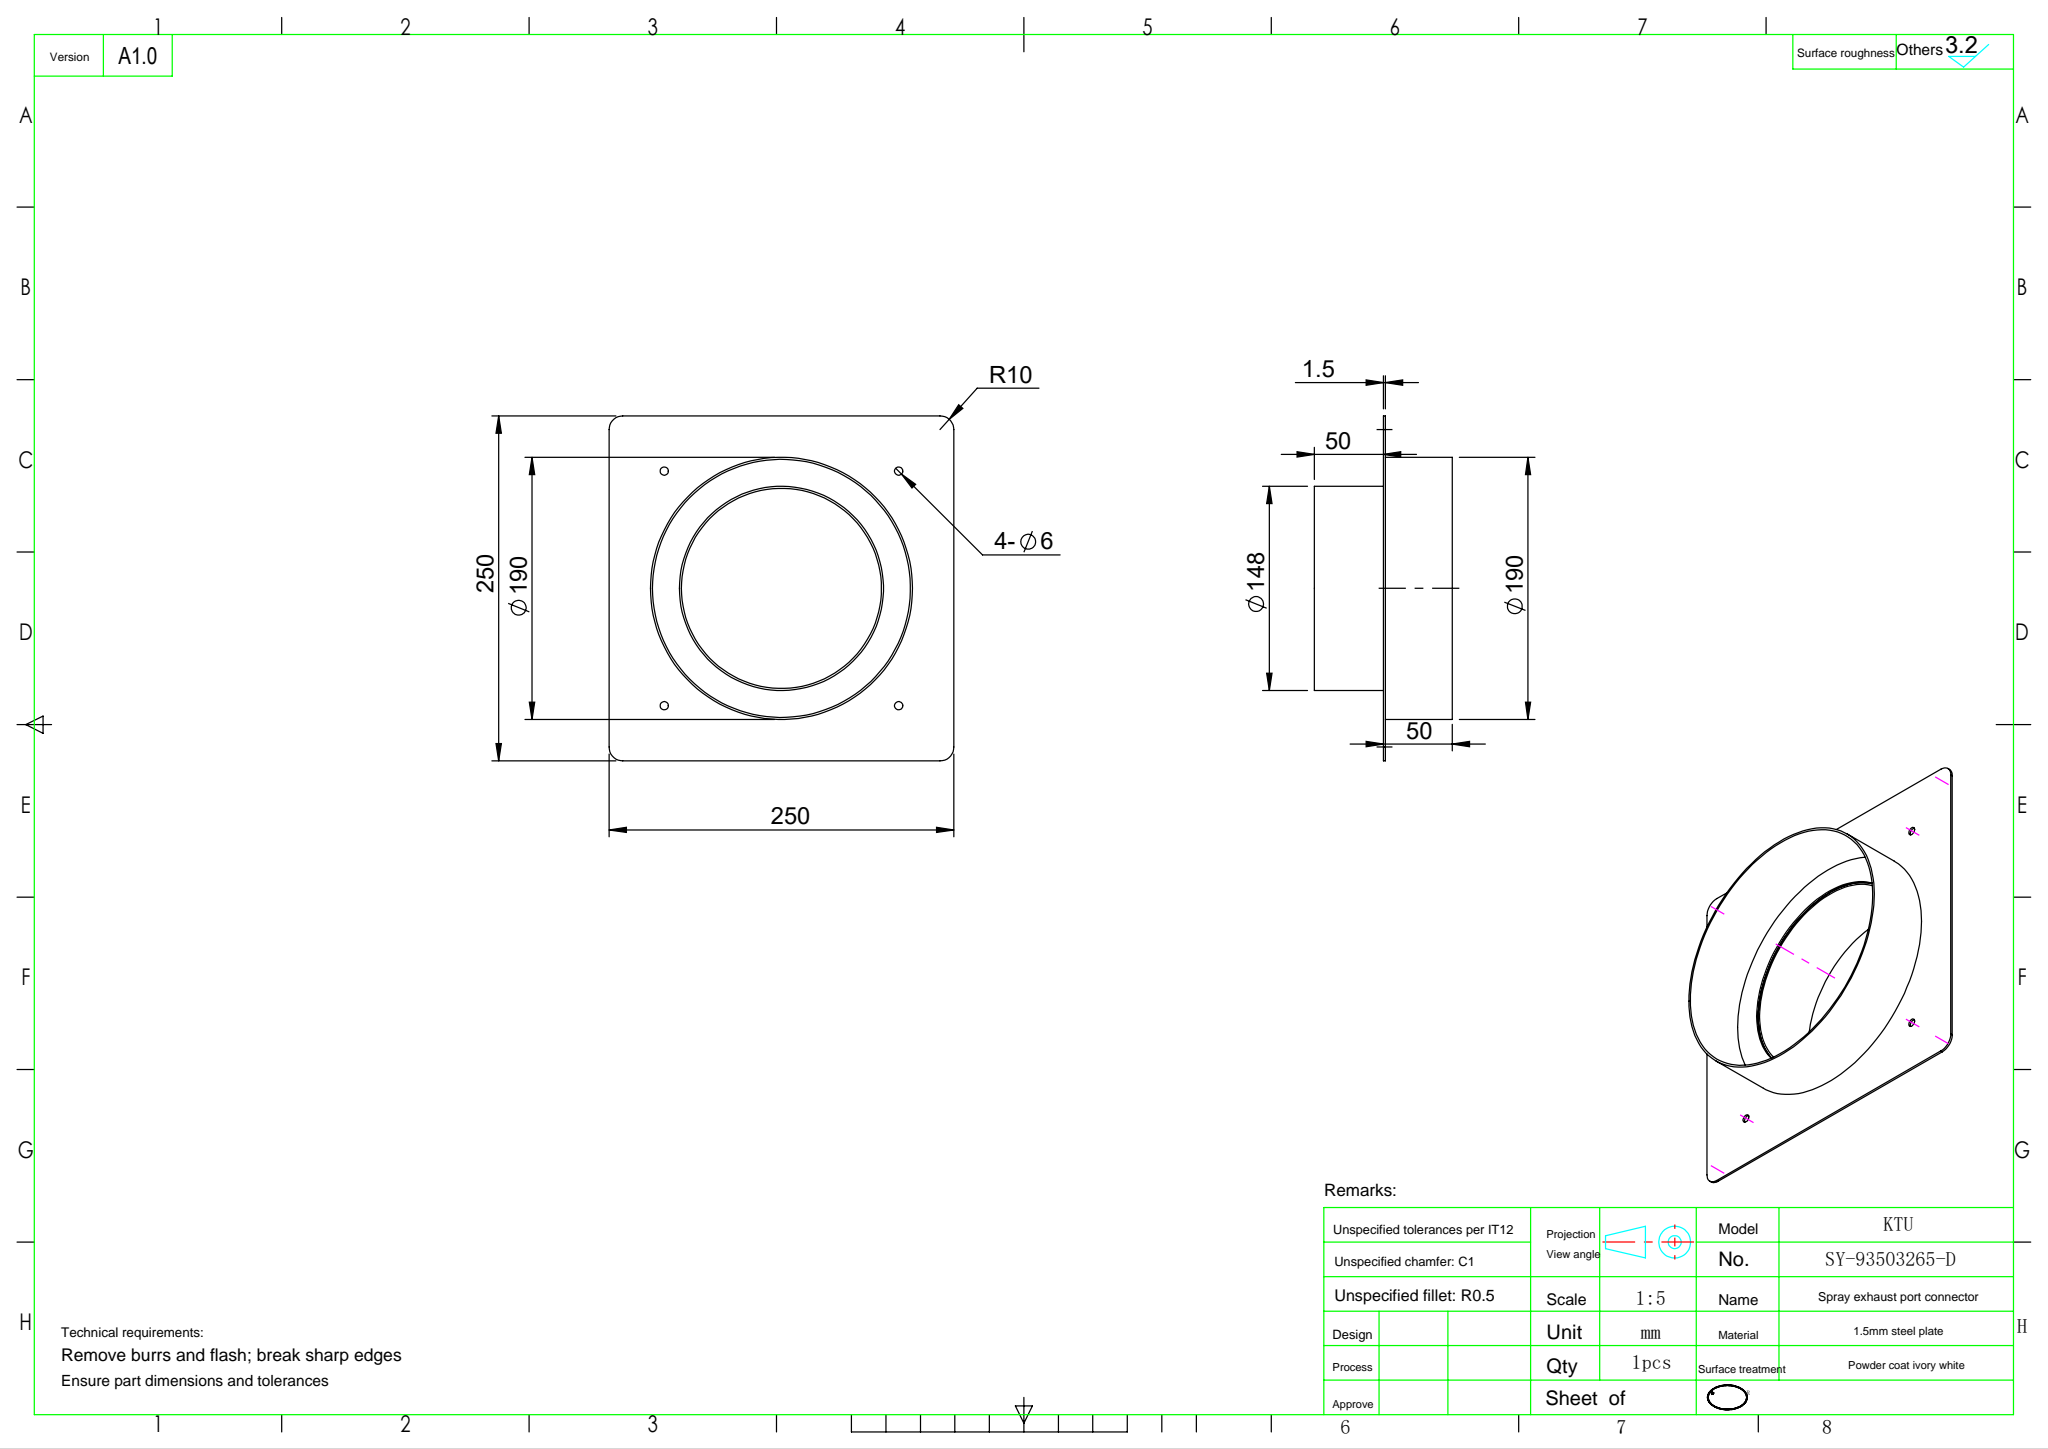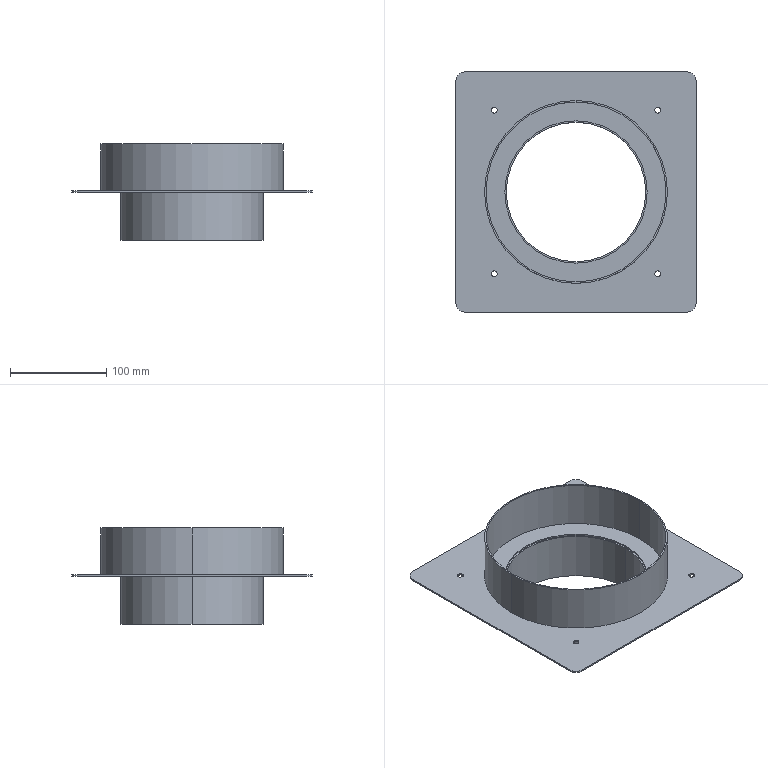Part | SolidWorks | features ICE 4, FlatPattern 1, SMBaseFlange 1, SheetMetal 1 | 2 solids | 32 faces | box 250 x 250 x 100 mm | volume 145247 mm3 | cylinder 22 | plane 10 | commonest cylinder face diameters 6 x8 20 x4 148 x4 145 x2 187 x2 190 x2
STEP:
#1=CARTESIAN_POINT('',(74.,0.,0.));
#2=VERTEX_POINT('',#1);
#3=CARTESIAN_POINT('',(-74.,0.,0.));
#4=VERTEX_POINT('',#3);
#5=CARTESIAN_POINT('',(0.,0.,0.));
#6=DIRECTION('',(0.,0.,-1.));
#7=DIRECTION('',(-1.,0.,0.));
#8=AXIS2_PLACEMENT_3D('',#5,#6,#7);
#9=CIRCLE('',#8,74.);
#10=EDGE_CURVE('',#2,#4,#9,.T.);
#11=ORIENTED_EDGE('',*,*,#10,.F.);
#12=CARTESIAN_POINT('',(74.,0.,-1.5));
#13=VERTEX_POINT('',#12);
#14=CARTESIAN_POINT('',(74.,0.,0.));
#15=DIRECTION('',(0.,0.,-1.));
#16=VECTOR('',#15,1000.);
#17=LINE('',#14,#16);
#18=EDGE_CURVE('',#2,#13,#17,.T.);
#19=ORIENTED_EDGE('',*,*,#18,.T.);
#20=CARTESIAN_POINT('',(-74.,0.,-1.5));
#21=VERTEX_POINT('',#20);
#22=CARTESIAN_POINT('',(0.,0.,-1.5));
#23=DIRECTION('',(0.,0.,-1.));
#24=DIRECTION('',(-1.,0.,0.));
#25=AXIS2_PLACEMENT_3D('',#22,#23,#24);
#26=CIRCLE('',#25,74.);
#27=EDGE_CURVE('',#13,#21,#26,.T.);
#28=ORIENTED_EDGE('',*,*,#27,.T.);
#29=CARTESIAN_POINT('',(-74.,0.,0.));
#30=DIRECTION('',(0.,0.,-1.));
#31=VECTOR('',#30,1000.);
#32=LINE('',#29,#31);
#33=EDGE_CURVE('',#4,#21,#32,.T.);
#34=ORIENTED_EDGE('',*,*,#33,.F.);
#35=EDGE_LOOP('',(#11,#19,#28,#34));
#36=FACE_OUTER_BOUND('',#35,.T.);
#37=CARTESIAN_POINT('',(0.,0.,0.));
#38=DIRECTION('',(0.,0.,-1.));
#39=DIRECTION('',(-1.,0.,0.));
#40=AXIS2_PLACEMENT_3D('',#37,#38,#39);
#41=CYLINDRICAL_SURFACE('',#40,74.);
#42=ADVANCED_FACE('',(#36),#41,.F.);
#43=CARTESIAN_POINT('',(82.,85.,0.));
#44=VERTEX_POINT('',#43);
#45=CARTESIAN_POINT('',(88.,85.,0.));
#46=VERTEX_POINT('',#45);
#47=CARTESIAN_POINT('',(85.,85.,0.));
#48=DIRECTION('',(0.,0.,1.));
#49=DIRECTION('',(1.,0.,0.));
#50=AXIS2_PLACEMENT_3D('',#47,#48,#49);
#51=CIRCLE('',#50,3.);
#52=EDGE_CURVE('',#44,#46,#51,.T.);
#53=ORIENTED_EDGE('',*,*,#52,.T.);
#54=CARTESIAN_POINT('',(88.,85.,-1.5));
#55=VERTEX_POINT('',#54);
#56=CARTESIAN_POINT('',(88.,85.,46.5));
#57=DIRECTION('',(0.,0.,-1.));
#58=VECTOR('',#57,1000.);
#59=LINE('',#56,#58);
#60=EDGE_CURVE('',#46,#55,#59,.T.);
#61=ORIENTED_EDGE('',*,*,#60,.T.);
#62=CARTESIAN_POINT('',(82.,85.,-1.5));
#63=VERTEX_POINT('',#62);
#64=CARTESIAN_POINT('',(85.,85.,-1.5));
#65=DIRECTION('',(0.,0.,-1.));
#66=DIRECTION('',(-1.,0.,0.));
#67=AXIS2_PLACEMENT_3D('',#64,#65,#66);
#68=CIRCLE('',#67,3.);
#69=EDGE_CURVE('',#55,#63,#68,.T.);
#70=ORIENTED_EDGE('',*,*,#69,.T.);
#71=CARTESIAN_POINT('',(82.,85.,46.5));
#72=DIRECTION('',(0.,0.,-1.));
#73=VECTOR('',#72,1000.);
#74=LINE('',#71,#73);
#75=EDGE_CURVE('',#44,#63,#74,.T.);
#76=ORIENTED_EDGE('',*,*,#75,.F.);
#77=EDGE_LOOP('',(#53,#61,#70,#76));
#78=FACE_OUTER_BOUND('',#77,.T.);
#79=CARTESIAN_POINT('',(85.,85.,46.5));
#80=DIRECTION('',(0.,0.,-1.));
#81=DIRECTION('',(-1.,0.,0.));
#82=AXIS2_PLACEMENT_3D('',#79,#80,#81);
#83=CYLINDRICAL_SURFACE('',#82,3.);
#84=ADVANCED_FACE('',(#78),#83,.F.);
#85=CARTESIAN_POINT('',(82.,-85.,0.));
#86=VERTEX_POINT('',#85);
#87=CARTESIAN_POINT('',(88.,-85.,0.));
#88=VERTEX_POINT('',#87);
#89=CARTESIAN_POINT('',(85.,-85.,0.));
#90=DIRECTION('',(0.,0.,1.));
#91=DIRECTION('',(1.,0.,0.));
#92=AXIS2_PLACEMENT_3D('',#89,#90,#91);
#93=CIRCLE('',#92,3.);
#94=EDGE_CURVE('',#86,#88,#93,.T.);
#95=ORIENTED_EDGE('',*,*,#94,.T.);
#96=CARTESIAN_POINT('',(88.,-85.,-1.5));
#97=VERTEX_POINT('',#96);
#98=CARTESIAN_POINT('',(88.,-85.,46.5));
#99=DIRECTION('',(0.,0.,-1.));
#100=VECTOR('',#99,1000.);
#101=LINE('',#98,#100);
#102=EDGE_CURVE('',#88,#97,#101,.T.);
#103=ORIENTED_EDGE('',*,*,#102,.T.);
#104=CARTESIAN_POINT('',(82.,-85.,-1.5));
#105=VERTEX_POINT('',#104);
#106=CARTESIAN_POINT('',(85.,-85.,-1.5));
#107=DIRECTION('',(0.,0.,-1.));
#108=DIRECTION('',(-1.,0.,0.));
#109=AXIS2_PLACEMENT_3D('',#106,#107,#108);
#110=CIRCLE('',#109,3.);
#111=EDGE_CURVE('',#97,#105,#110,.T.);
#112=ORIENTED_EDGE('',*,*,#111,.T.);
#113=CARTESIAN_POINT('',(82.,-85.,46.5));
#114=DIRECTION('',(0.,0.,-1.));
#115=VECTOR('',#114,1000.);
#116=LINE('',#113,#115);
#117=EDGE_CURVE('',#86,#105,#116,.T.);
#118=ORIENTED_EDGE('',*,*,#117,.F.);
#119=EDGE_LOOP('',(#95,#103,#112,#118));
#120=FACE_OUTER_BOUND('',#119,.T.);
#121=CARTESIAN_POINT('',(85.,-85.,46.5));
#122=DIRECTION('',(0.,0.,-1.));
#123=DIRECTION('',(-1.,0.,0.));
#124=AXIS2_PLACEMENT_3D('',#121,#122,#123);
#125=CYLINDRICAL_SURFACE('',#124,3.);
#126=ADVANCED_FACE('',(#120),#125,.F.);
#127=CARTESIAN_POINT('',(-88.,-85.,0.));
#128=VERTEX_POINT('',#127);
#129=CARTESIAN_POINT('',(-82.,-85.,0.));
#130=VERTEX_POINT('',#129);
#131=CARTESIAN_POINT('',(-85.,-85.,0.));
#132=DIRECTION('',(0.,0.,1.));
#133=DIRECTION('',(1.,0.,0.));
#134=AXIS2_PLACEMENT_3D('',#131,#132,#133);
#135=CIRCLE('',#134,3.);
#136=EDGE_CURVE('',#128,#130,#135,.T.);
#137=ORIENTED_EDGE('',*,*,#136,.T.);
#138=CARTESIAN_POINT('',(-82.,-85.,-1.5));
#139=VERTEX_POINT('',#138);
#140=CARTESIAN_POINT('',(-82.,-85.,46.5));
#141=DIRECTION('',(0.,0.,-1.));
#142=VECTOR('',#141,1000.);
#143=LINE('',#140,#142);
#144=EDGE_CURVE('',#130,#139,#143,.T.);
#145=ORIENTED_EDGE('',*,*,#144,.T.);
#146=CARTESIAN_POINT('',(-88.,-85.,-1.5));
#147=VERTEX_POINT('',#146);
#148=CARTESIAN_POINT('',(-85.,-85.,-1.5));
#149=DIRECTION('',(0.,0.,-1.));
#150=DIRECTION('',(-1.,0.,0.));
#151=AXIS2_PLACEMENT_3D('',#148,#149,#150);
#152=CIRCLE('',#151,3.);
#153=EDGE_CURVE('',#139,#147,#152,.T.);
#154=ORIENTED_EDGE('',*,*,#153,.T.);
#155=CARTESIAN_POINT('',(-88.,-85.,46.5));
#156=DIRECTION('',(0.,0.,-1.));
#157=VECTOR('',#156,1000.);
#158=LINE('',#155,#157);
#159=EDGE_CURVE('',#128,#147,#158,.T.);
#160=ORIENTED_EDGE('',*,*,#159,.F.);
#161=EDGE_LOOP('',(#137,#145,#154,#160));
#162=FACE_OUTER_BOUND('',#161,.T.);
#163=CARTESIAN_POINT('',(-85.,-85.,46.5));
#164=DIRECTION('',(0.,0.,-1.));
#165=DIRECTION('',(-1.,0.,0.));
#166=AXIS2_PLACEMENT_3D('',#163,#164,#165);
#167=CYLINDRICAL_SURFACE('',#166,3.);
#168=ADVANCED_FACE('',(#162),#167,.F.);
#169=CARTESIAN_POINT('',(-88.,85.,0.));
#170=VERTEX_POINT('',#169);
#171=CARTESIAN_POINT('',(-82.,85.,0.));
#172=VERTEX_POINT('',#171);
#173=CARTESIAN_POINT('',(-85.,85.,0.));
#174=DIRECTION('',(0.,0.,1.));
#175=DIRECTION('',(1.,0.,0.));
#176=AXIS2_PLACEMENT_3D('',#173,#174,#175);
#177=CIRCLE('',#176,3.);
#178=EDGE_CURVE('',#170,#172,#177,.T.);
#179=ORIENTED_EDGE('',*,*,#178,.T.);
#180=CARTESIAN_POINT('',(-82.,85.,-1.5));
#181=VERTEX_POINT('',#180);
#182=CARTESIAN_POINT('',(-82.,85.,46.5));
#183=DIRECTION('',(0.,0.,-1.));
#184=VECTOR('',#183,1000.);
#185=LINE('',#182,#184);
#186=EDGE_CURVE('',#172,#181,#185,.T.);
#187=ORIENTED_EDGE('',*,*,#186,.T.);
#188=CARTESIAN_POINT('',(-88.,85.,-1.5));
#189=VERTEX_POINT('',#188);
#190=CARTESIAN_POINT('',(-85.,85.,-1.5));
#191=DIRECTION('',(0.,0.,-1.));
#192=DIRECTION('',(-1.,0.,0.));
#193=AXIS2_PLACEMENT_3D('',#190,#191,#192);
#194=CIRCLE('',#193,3.);
#195=EDGE_CURVE('',#181,#189,#194,.T.);
#196=ORIENTED_EDGE('',*,*,#195,.T.);
#197=CARTESIAN_POINT('',(-88.,85.,46.5));
#198=DIRECTION('',(0.,0.,-1.));
#199=VECTOR('',#198,1000.);
#200=LINE('',#197,#199);
#201=EDGE_CURVE('',#170,#189,#200,.T.);
#202=ORIENTED_EDGE('',*,*,#201,.F.);
#203=EDGE_LOOP('',(#179,#187,#196,#202));
#204=FACE_OUTER_BOUND('',#203,.T.);
#205=CARTESIAN_POINT('',(-85.,85.,46.5));
#206=DIRECTION('',(0.,0.,-1.));
#207=DIRECTION('',(-1.,0.,0.));
#208=AXIS2_PLACEMENT_3D('',#205,#206,#207);
#209=CYLINDRICAL_SURFACE('',#208,3.);
#210=ADVANCED_FACE('',(#204),#209,.F.);
#211=CARTESIAN_POINT('',(-95.,0.,48.5));
#212=VERTEX_POINT('',#211);
#213=CARTESIAN_POINT('',(95.,0.,48.5));
#214=VERTEX_POINT('',#213);
#215=CARTESIAN_POINT('',(0.,0.,48.5));
#216=DIRECTION('',(0.,0.,-1.));
#217=DIRECTION('',(-1.,0.,0.));
#218=AXIS2_PLACEMENT_3D('',#215,#216,#217);
#219=CIRCLE('',#218,95.);
#220=EDGE_CURVE('',#212,#214,#219,.T.);
#221=ORIENTED_EDGE('',*,*,#220,.T.);
#222=CARTESIAN_POINT('',(95.,0.,0.));
#223=VERTEX_POINT('',#222);
#224=CARTESIAN_POINT('',(95.,0.,48.5));
#225=DIRECTION('',(0.,0.,-1.));
#226=VECTOR('',#225,1000.);
#227=LINE('',#224,#226);
#228=EDGE_CURVE('',#214,#223,#227,.T.);
#229=ORIENTED_EDGE('',*,*,#228,.T.);
#230=CARTESIAN_POINT('',(-95.,0.,0.));
#231=VERTEX_POINT('',#230);
#232=CARTESIAN_POINT('',(0.,0.,0.));
#233=DIRECTION('',(0.,0.,1.));
#234=DIRECTION('',(1.,0.,0.));
#235=AXIS2_PLACEMENT_3D('',#232,#233,#234);
#236=CIRCLE('',#235,95.);
#237=EDGE_CURVE('',#223,#231,#236,.T.);
#238=ORIENTED_EDGE('',*,*,#237,.T.);
#239=CARTESIAN_POINT('',(-95.,0.,48.5));
#240=DIRECTION('',(0.,0.,-1.));
#241=VECTOR('',#240,1000.);
#242=LINE('',#239,#241);
#243=EDGE_CURVE('',#212,#231,#242,.T.);
#244=ORIENTED_EDGE('',*,*,#243,.F.);
#245=EDGE_LOOP('',(#221,#229,#238,#244));
#246=FACE_OUTER_BOUND('',#245,.T.);
#247=CARTESIAN_POINT('',(0.,0.,48.5));
#248=DIRECTION('',(0.,0.,-1.));
#249=DIRECTION('',(-1.,0.,0.));
#250=AXIS2_PLACEMENT_3D('',#247,#248,#249);
#251=CYLINDRICAL_SURFACE('',#250,95.);
#252=ADVANCED_FACE('',(#246),#251,.T.);
#253=CARTESIAN_POINT('',(93.5,0.,48.5));
#254=VERTEX_POINT('',#253);
#255=CARTESIAN_POINT('',(-93.5,0.,48.5));
#256=VERTEX_POINT('',#255);
#257=CARTESIAN_POINT('',(0.,0.,48.5));
#258=DIRECTION('',(0.,0.,-1.));
#259=DIRECTION('',(-1.,0.,0.));
#260=AXIS2_PLACEMENT_3D('',#257,#258,#259);
#261=CIRCLE('',#260,93.5);
#262=EDGE_CURVE('',#254,#256,#261,.T.);
#263=ORIENTED_EDGE('',*,*,#262,.F.);
#264=CARTESIAN_POINT('',(93.5,0.,0.));
#265=VERTEX_POINT('',#264);
#266=CARTESIAN_POINT('',(93.5,0.,48.5));
#267=DIRECTION('',(0.,0.,-1.));
#268=VECTOR('',#267,1000.);
#269=LINE('',#266,#268);
#270=EDGE_CURVE('',#254,#265,#269,.T.);
#271=ORIENTED_EDGE('',*,*,#270,.T.);
#272=CARTESIAN_POINT('',(-93.5,0.,0.));
#273=VERTEX_POINT('',#272);
#274=CARTESIAN_POINT('',(0.,0.,0.));
#275=DIRECTION('',(0.,0.,1.));
#276=DIRECTION('',(-1.,0.,0.));
#277=AXIS2_PLACEMENT_3D('',#274,#275,#276);
#278=CIRCLE('',#277,93.5);
#279=EDGE_CURVE('',#273,#265,#278,.T.);
#280=ORIENTED_EDGE('',*,*,#279,.F.);
#281=CARTESIAN_POINT('',(-93.5,0.,48.5));
#282=DIRECTION('',(0.,0.,-1.));
#283=VECTOR('',#282,1000.);
#284=LINE('',#281,#283);
#285=EDGE_CURVE('',#256,#273,#284,.T.);
#286=ORIENTED_EDGE('',*,*,#285,.F.);
#287=EDGE_LOOP('',(#263,#271,#280,#286));
#288=FACE_OUTER_BOUND('',#287,.T.);
#289=CARTESIAN_POINT('',(0.,0.,48.5));
#290=DIRECTION('',(0.,0.,-1.));
#291=DIRECTION('',(-1.,0.,0.));
#292=AXIS2_PLACEMENT_3D('',#289,#290,#291);
#293=CYLINDRICAL_SURFACE('',#292,93.5);
#294=ADVANCED_FACE('',(#288),#293,.F.);
#295=ORIENTED_EDGE('',*,*,#270,.F.);
#296=CARTESIAN_POINT('',(0.,0.,48.5));
#297=DIRECTION('',(0.,0.,-1.));
#298=DIRECTION('',(-1.,0.,0.));
#299=AXIS2_PLACEMENT_3D('',#296,#297,#298);
#300=CIRCLE('',#299,93.5);
#301=EDGE_CURVE('',#256,#254,#300,.T.);
#302=ORIENTED_EDGE('',*,*,#301,.F.);
#303=ORIENTED_EDGE('',*,*,#285,.T.);
#304=CARTESIAN_POINT('',(0.,0.,0.));
#305=DIRECTION('',(0.,0.,1.));
#306=DIRECTION('',(-1.,0.,0.));
#307=AXIS2_PLACEMENT_3D('',#304,#305,#306);
#308=CIRCLE('',#307,93.5);
#309=EDGE_CURVE('',#265,#273,#308,.T.);
#310=ORIENTED_EDGE('',*,*,#309,.F.);
#311=EDGE_LOOP('',(#295,#302,#303,#310));
#312=FACE_OUTER_BOUND('',#311,.T.);
#313=CARTESIAN_POINT('',(0.,0.,48.5));
#314=DIRECTION('',(0.,0.,-1.));
#315=DIRECTION('',(-1.,0.,0.));
#316=AXIS2_PLACEMENT_3D('',#313,#314,#315);
#317=CYLINDRICAL_SURFACE('',#316,93.5);
#318=ADVANCED_FACE('',(#312),#317,.F.);
#319=CARTESIAN_POINT('',(-125.,-115.,0.));
#320=VERTEX_POINT('',#319);
#321=CARTESIAN_POINT('',(-115.,-125.,0.));
#322=VERTEX_POINT('',#321);
#323=CARTESIAN_POINT('',(-115.,-115.,0.));
#324=DIRECTION('',(0.,0.,1.));
#325=DIRECTION('',(1.,0.,0.));
#326=AXIS2_PLACEMENT_3D('',#323,#324,#325);
#327=CIRCLE('',#326,10.);
#328=EDGE_CURVE('',#320,#322,#327,.T.);
#329=ORIENTED_EDGE('',*,*,#328,.F.);
#330=CARTESIAN_POINT('',(-125.,-115.,-1.5));
#331=VERTEX_POINT('',#330);
#332=CARTESIAN_POINT('',(-125.,-115.,-1.5));
#333=DIRECTION('',(0.,0.,1.));
#334=VECTOR('',#333,1000.);
#335=LINE('',#332,#334);
#336=EDGE_CURVE('',#331,#320,#335,.T.);
#337=ORIENTED_EDGE('',*,*,#336,.F.);
#338=CARTESIAN_POINT('',(-115.,-125.,-1.5));
#339=VERTEX_POINT('',#338);
#340=CARTESIAN_POINT('',(-115.,-115.,-1.5));
#341=DIRECTION('',(0.,0.,1.));
#342=DIRECTION('',(1.,0.,0.));
#343=AXIS2_PLACEMENT_3D('',#340,#341,#342);
#344=CIRCLE('',#343,10.);
#345=EDGE_CURVE('',#331,#339,#344,.T.);
#346=ORIENTED_EDGE('',*,*,#345,.T.);
#347=CARTESIAN_POINT('',(-115.,-125.,-1.5));
#348=DIRECTION('',(0.,0.,1.));
#349=VECTOR('',#348,1000.);
#350=LINE('',#347,#349);
#351=EDGE_CURVE('',#339,#322,#350,.T.);
#352=ORIENTED_EDGE('',*,*,#351,.T.);
#353=EDGE_LOOP('',(#329,#337,#346,#352));
#354=FACE_OUTER_BOUND('',#353,.T.);
#355=CARTESIAN_POINT('',(-115.,-115.,-1.5));
#356=DIRECTION('',(0.,0.,1.));
#357=DIRECTION('',(1.,0.,0.));
#358=AXIS2_PLACEMENT_3D('',#355,#356,#357);
#359=CYLINDRICAL_SURFACE('',#358,10.);
#360=ADVANCED_FACE('',(#354),#359,.T.);
#361=CARTESIAN_POINT('',(-125.,115.,0.));
#362=VERTEX_POINT('',#361);
#363=CARTESIAN_POINT('',(-125.,-115.,0.));
#364=DIRECTION('',(0.,-1.,0.));
#365=VECTOR('',#364,1000.);
#366=LINE('',#363,#365);
#367=EDGE_CURVE('',#362,#320,#366,.T.);
#368=ORIENTED_EDGE('',*,*,#367,.F.);
#369=CARTESIAN_POINT('',(-125.,115.,-1.5));
#370=VERTEX_POINT('',#369);
#371=CARTESIAN_POINT('',(-125.,115.,-1.5));
#372=DIRECTION('',(0.,0.,1.));
#373=VECTOR('',#372,1000.);
#374=LINE('',#371,#373);
#375=EDGE_CURVE('',#370,#362,#374,.T.);
#376=ORIENTED_EDGE('',*,*,#375,.F.);
#377=CARTESIAN_POINT('',(-125.,-115.,-1.5));
#378=DIRECTION('',(0.,-1.,0.));
#379=VECTOR('',#378,1000.);
#380=LINE('',#377,#379);
#381=EDGE_CURVE('',#370,#331,#380,.T.);
#382=ORIENTED_EDGE('',*,*,#381,.T.);
#383=ORIENTED_EDGE('',*,*,#336,.T.);
#384=EDGE_LOOP('',(#368,#376,#382,#383));
#385=FACE_OUTER_BOUND('',#384,.T.);
#386=CARTESIAN_POINT('',(-125.,-115.,-1.5));
#387=DIRECTION('',(-1.,0.,0.));
#388=DIRECTION('',(0.,0.,1.));
#389=AXIS2_PLACEMENT_3D('',#386,#387,#388);
#390=PLANE('',#389);
#391=ADVANCED_FACE('',(#385),#390,.T.);
#392=CARTESIAN_POINT('',(-115.,125.,0.));
#393=VERTEX_POINT('',#392);
#394=CARTESIAN_POINT('',(-115.,115.,0.));
#395=DIRECTION('',(0.,0.,1.));
#396=DIRECTION('',(-1.,0.,0.));
#397=AXIS2_PLACEMENT_3D('',#394,#395,#396);
#398=CIRCLE('',#397,10.);
#399=EDGE_CURVE('',#393,#362,#398,.T.);
#400=ORIENTED_EDGE('',*,*,#399,.F.);
#401=CARTESIAN_POINT('',(-115.,125.,-1.5));
#402=VERTEX_POINT('',#401);
#403=CARTESIAN_POINT('',(-115.,125.,-1.5));
#404=DIRECTION('',(0.,0.,1.));
#405=VECTOR('',#404,1000.);
#406=LINE('',#403,#405);
#407=EDGE_CURVE('',#402,#393,#406,.T.);
#408=ORIENTED_EDGE('',*,*,#407,.F.);
#409=CARTESIAN_POINT('',(-115.,115.,-1.5));
#410=DIRECTION('',(0.,0.,1.));
#411=DIRECTION('',(-1.,0.,0.));
#412=AXIS2_PLACEMENT_3D('',#409,#410,#411);
#413=CIRCLE('',#412,10.);
#414=EDGE_CURVE('',#402,#370,#413,.T.);
#415=ORIENTED_EDGE('',*,*,#414,.T.);
#416=ORIENTED_EDGE('',*,*,#375,.T.);
#417=EDGE_LOOP('',(#400,#408,#415,#416));
#418=FACE_OUTER_BOUND('',#417,.T.);
#419=CARTESIAN_POINT('',(-115.,115.,-1.5));
#420=DIRECTION('',(0.,0.,1.));
#421=DIRECTION('',(1.,0.,0.));
#422=AXIS2_PLACEMENT_3D('',#419,#420,#421);
#423=CYLINDRICAL_SURFACE('',#422,10.);
#424=ADVANCED_FACE('',(#418),#423,.T.);
#425=CARTESIAN_POINT('',(115.,125.,0.));
#426=VERTEX_POINT('',#425);
#427=CARTESIAN_POINT('',(-115.,125.,0.));
#428=DIRECTION('',(-1.,0.,0.));
#429=VECTOR('',#428,1000.);
#430=LINE('',#427,#429);
#431=EDGE_CURVE('',#426,#393,#430,.T.);
#432=ORIENTED_EDGE('',*,*,#431,.F.);
#433=CARTESIAN_POINT('',(115.,125.,-1.5));
#434=VERTEX_POINT('',#433);
#435=CARTESIAN_POINT('',(115.,125.,-1.5));
#436=DIRECTION('',(0.,0.,1.));
#437=VECTOR('',#436,1000.);
#438=LINE('',#435,#437);
#439=EDGE_CURVE('',#434,#426,#438,.T.);
#440=ORIENTED_EDGE('',*,*,#439,.F.);
#441=CARTESIAN_POINT('',(-115.,125.,-1.5));
#442=DIRECTION('',(-1.,0.,0.));
#443=VECTOR('',#442,1000.);
#444=LINE('',#441,#443);
#445=EDGE_CURVE('',#434,#402,#444,.T.);
#446=ORIENTED_EDGE('',*,*,#445,.T.);
#447=ORIENTED_EDGE('',*,*,#407,.T.);
#448=EDGE_LOOP('',(#432,#440,#446,#447));
#449=FACE_OUTER_BOUND('',#448,.T.);
#450=CARTESIAN_POINT('',(-115.,125.,-1.5));
#451=DIRECTION('',(0.,1.,0.));
#452=DIRECTION('',(0.,0.,1.));
#453=AXIS2_PLACEMENT_3D('',#450,#451,#452);
#454=PLANE('',#453);
#455=ADVANCED_FACE('',(#449),#454,.T.);
#456=CARTESIAN_POINT('',(125.,115.,0.));
#457=VERTEX_POINT('',#456);
#458=CARTESIAN_POINT('',(115.,115.,0.));
#459=DIRECTION('',(0.,0.,1.));
#460=DIRECTION('',(1.,0.,0.));
#461=AXIS2_PLACEMENT_3D('',#458,#459,#460);
#462=CIRCLE('',#461,10.);
#463=EDGE_CURVE('',#457,#426,#462,.T.);
#464=ORIENTED_EDGE('',*,*,#463,.F.);
#465=CARTESIAN_POINT('',(125.,115.,-1.5));
#466=VERTEX_POINT('',#465);
#467=CARTESIAN_POINT('',(125.,115.,-1.5));
#468=DIRECTION('',(0.,0.,1.));
#469=VECTOR('',#468,1000.);
#470=LINE('',#467,#469);
#471=EDGE_CURVE('',#466,#457,#470,.T.);
#472=ORIENTED_EDGE('',*,*,#471,.F.);
#473=CARTESIAN_POINT('',(115.,115.,-1.5));
#474=DIRECTION('',(0.,0.,1.));
#475=DIRECTION('',(1.,0.,0.));
#476=AXIS2_PLACEMENT_3D('',#473,#474,#475);
#477=CIRCLE('',#476,10.);
#478=EDGE_CURVE('',#466,#434,#477,.T.);
#479=ORIENTED_EDGE('',*,*,#478,.T.);
#480=ORIENTED_EDGE('',*,*,#439,.T.);
#481=EDGE_LOOP('',(#464,#472,#479,#480));
#482=FACE_OUTER_BOUND('',#481,.T.);
#483=CARTESIAN_POINT('',(115.,115.,-1.5));
#484=DIRECTION('',(0.,0.,1.));
#485=DIRECTION('',(1.,0.,0.));
#486=AXIS2_PLACEMENT_3D('',#483,#484,#485);
#487=CYLINDRICAL_SURFACE('',#486,10.);
#488=ADVANCED_FACE('',(#482),#487,.T.);
#489=CARTESIAN_POINT('',(125.,-115.,0.));
#490=VERTEX_POINT('',#489);
#491=CARTESIAN_POINT('',(125.,-115.,0.));
#492=DIRECTION('',(0.,1.,0.));
#493=VECTOR('',#492,1000.);
#494=LINE('',#491,#493);
#495=EDGE_CURVE('',#490,#457,#494,.T.);
#496=ORIENTED_EDGE('',*,*,#495,.F.);
#497=CARTESIAN_POINT('',(125.,-115.,-1.5));
#498=VERTEX_POINT('',#497);
#499=CARTESIAN_POINT('',(125.,-115.,-1.5));
#500=DIRECTION('',(0.,0.,1.));
#501=VECTOR('',#500,1000.);
#502=LINE('',#499,#501);
#503=EDGE_CURVE('',#498,#490,#502,.T.);
#504=ORIENTED_EDGE('',*,*,#503,.F.);
#505=CARTESIAN_POINT('',(125.,-115.,-1.5));
#506=DIRECTION('',(0.,1.,0.));
#507=VECTOR('',#506,1000.);
#508=LINE('',#505,#507);
#509=EDGE_CURVE('',#498,#466,#508,.T.);
#510=ORIENTED_EDGE('',*,*,#509,.T.);
#511=ORIENTED_EDGE('',*,*,#471,.T.);
#512=EDGE_LOOP('',(#496,#504,#510,#511));
#513=FACE_OUTER_BOUND('',#512,.T.);
#514=CARTESIAN_POINT('',(125.,-115.,-1.5));
#515=DIRECTION('',(1.,0.,0.));
#516=DIRECTION('',(0.,0.,-1.));
#517=AXIS2_PLACEMENT_3D('',#514,#515,#516);
#518=PLANE('',#517);
#519=ADVANCED_FACE('',(#513),#518,.T.);
#520=CARTESIAN_POINT('',(115.,-125.,0.));
#521=VERTEX_POINT('',#520);
#522=CARTESIAN_POINT('',(115.,-115.,0.));
#523=DIRECTION('',(0.,0.,1.));
#524=DIRECTION('',(1.,0.,0.));
#525=AXIS2_PLACEMENT_3D('',#522,#523,#524);
#526=CIRCLE('',#525,10.);
#527=EDGE_CURVE('',#521,#490,#526,.T.);
#528=ORIENTED_EDGE('',*,*,#527,.F.);
#529=CARTESIAN_POINT('',(115.,-125.,-1.5));
#530=VERTEX_POINT('',#529);
#531=CARTESIAN_POINT('',(115.,-125.,-1.5));
#532=DIRECTION('',(0.,0.,1.));
#533=VECTOR('',#532,1000.);
#534=LINE('',#531,#533);
#535=EDGE_CURVE('',#530,#521,#534,.T.);
#536=ORIENTED_EDGE('',*,*,#535,.F.);
#537=CARTESIAN_POINT('',(115.,-115.,-1.5));
#538=DIRECTION('',(0.,0.,1.));
#539=DIRECTION('',(1.,0.,0.));
#540=AXIS2_PLACEMENT_3D('',#537,#538,#539);
#541=CIRCLE('',#540,10.);
#542=EDGE_CURVE('',#530,#498,#541,.T.);
#543=ORIENTED_EDGE('',*,*,#542,.T.);
#544=ORIENTED_EDGE('',*,*,#503,.T.);
#545=EDGE_LOOP('',(#528,#536,#543,#544));
#546=FACE_OUTER_BOUND('',#545,.T.);
#547=CARTESIAN_POINT('',(115.,-115.,-1.5));
#548=DIRECTION('',(0.,0.,1.));
#549=DIRECTION('',(1.,0.,0.));
#550=AXIS2_PLACEMENT_3D('',#547,#548,#549);
#551=CYLINDRICAL_SURFACE('',#550,10.);
#552=ADVANCED_FACE('',(#546),#551,.T.);
#553=CARTESIAN_POINT('',(-115.,-125.,0.));
#554=DIRECTION('',(1.,0.,0.));
#555=VECTOR('',#554,1000.);
#556=LINE('',#553,#555);
#557=EDGE_CURVE('',#322,#521,#556,.T.);
#558=ORIENTED_EDGE('',*,*,#557,.F.);
#559=ORIENTED_EDGE('',*,*,#351,.F.);
#560=CARTESIAN_POINT('',(-115.,-125.,-1.5));
#561=DIRECTION('',(1.,0.,0.));
#562=VECTOR('',#561,1000.);
#563=LINE('',#560,#562);
#564=EDGE_CURVE('',#339,#530,#563,.T.);
#565=ORIENTED_EDGE('',*,*,#564,.T.);
#566=ORIENTED_EDGE('',*,*,#535,.T.);
#567=EDGE_LOOP('',(#558,#559,#565,#566));
#568=FACE_OUTER_BOUND('',#567,.T.);
#569=CARTESIAN_POINT('',(-115.,-125.,-1.5));
#570=DIRECTION('',(0.,-1.,0.));
#571=DIRECTION('',(0.,0.,-1.));
#572=AXIS2_PLACEMENT_3D('',#569,#570,#571);
#573=PLANE('',#572);
#574=ADVANCED_FACE('',(#568),#573,.T.);
#575=CARTESIAN_POINT('',(85.,85.,-1.5));
#576=DIRECTION('',(0.,0.,-1.));
#577=DIRECTION('',(-1.,0.,0.));
#578=AXIS2_PLACEMENT_3D('',#575,#576,#577);
#579=CIRCLE('',#578,3.);
#580=EDGE_CURVE('',#63,#55,#579,.T.);
#581=ORIENTED_EDGE('',*,*,#580,.F.);
#582=ORIENTED_EDGE('',*,*,#69,.F.);
#583=EDGE_LOOP('',(#581,#582));
#584=FACE_BOUND('',#583,.T.);
#585=CARTESIAN_POINT('',(85.,-85.,-1.5));
#586=DIRECTION('',(0.,0.,-1.));
#587=DIRECTION('',(-1.,0.,0.));
#588=AXIS2_PLACEMENT_3D('',#585,#586,#587);
#589=CIRCLE('',#588,3.);
#590=EDGE_CURVE('',#105,#97,#589,.T.);
#591=ORIENTED_EDGE('',*,*,#590,.F.);
#592=ORIENTED_EDGE('',*,*,#111,.F.);
#593=EDGE_LOOP('',(#591,#592));
#594=FACE_BOUND('',#593,.T.);
#595=CARTESIAN_POINT('',(-85.,-85.,-1.5));
#596=DIRECTION('',(0.,0.,-1.));
#597=DIRECTION('',(-1.,0.,0.));
#598=AXIS2_PLACEMENT_3D('',#595,#596,#597);
#599=CIRCLE('',#598,3.);
#600=EDGE_CURVE('',#147,#139,#599,.T.);
#601=ORIENTED_EDGE('',*,*,#600,.F.);
#602=ORIENTED_EDGE('',*,*,#153,.F.);
#603=EDGE_LOOP('',(#601,#602));
#604=FACE_BOUND('',#603,.T.);
#605=CARTESIAN_POINT('',(-85.,85.,-1.5));
#606=DIRECTION('',(0.,0.,-1.));
#607=DIRECTION('',(-1.,0.,0.));
#608=AXIS2_PLACEMENT_3D('',#605,#606,#607);
#609=CIRCLE('',#608,3.);
#610=EDGE_CURVE('',#189,#181,#609,.T.);
#611=ORIENTED_EDGE('',*,*,#610,.F.);
#612=ORIENTED_EDGE('',*,*,#195,.F.);
#613=EDGE_LOOP('',(#611,#612));
#614=FACE_BOUND('',#613,.T.);
#615=ORIENTED_EDGE('',*,*,#345,.F.);
#616=ORIENTED_EDGE('',*,*,#381,.F.);
#617=ORIENTED_EDGE('',*,*,#414,.F.);
#618=ORIENTED_EDGE('',*,*,#445,.F.);
#619=ORIENTED_EDGE('',*,*,#478,.F.);
#620=ORIENTED_EDGE('',*,*,#509,.F.);
#621=ORIENTED_EDGE('',*,*,#542,.F.);
#622=ORIENTED_EDGE('',*,*,#564,.F.);
#623=EDGE_LOOP('',(#615,#616,#617,#618,#619,#620,#621,#622));
#624=FACE_OUTER_BOUND('',#623,.T.);
#625=CARTESIAN_POINT('',(0.,0.,-1.5));
#626=DIRECTION('',(0.,0.,-1.));
#627=DIRECTION('',(-1.,0.,0.));
#628=AXIS2_PLACEMENT_3D('',#625,#626,#627);
#629=CIRCLE('',#628,74.);
#630=EDGE_CURVE('',#21,#13,#629,.T.);
#631=ORIENTED_EDGE('',*,*,#630,.F.);
#632=ORIENTED_EDGE('',*,*,#27,.F.);
#633=EDGE_LOOP('',(#631,#632));
#634=FACE_BOUND('',#633,.T.);
#635=CARTESIAN_POINT('',(-115.,-115.,-1.5));
#636=DIRECTION('',(0.,0.,1.));
#637=DIRECTION('',(1.,0.,0.));
#638=AXIS2_PLACEMENT_3D('',#635,#636,#637);
#639=PLANE('',#638);
#640=ADVANCED_FACE('',(#584,#594,#604,#614,#624,#634),#639,.F.);
#641=ORIENTED_EDGE('',*,*,#52,.F.);
#642=CARTESIAN_POINT('',(85.,85.,0.));
#643=DIRECTION('',(0.,0.,1.));
#644=DIRECTION('',(1.,0.,0.));
#645=AXIS2_PLACEMENT_3D('',#642,#643,#644);
#646=CIRCLE('',#645,3.);
#647=EDGE_CURVE('',#46,#44,#646,.T.);
#648=ORIENTED_EDGE('',*,*,#647,.F.);
#649=EDGE_LOOP('',(#641,#648));
#650=FACE_BOUND('',#649,.T.);
#651=ORIENTED_EDGE('',*,*,#94,.F.);
#652=CARTESIAN_POINT('',(85.,-85.,0.));
#653=DIRECTION('',(0.,0.,1.));
#654=DIRECTION('',(1.,0.,0.));
#655=AXIS2_PLACEMENT_3D('',#652,#653,#654);
#656=CIRCLE('',#655,3.);
#657=EDGE_CURVE('',#88,#86,#656,.T.);
#658=ORIENTED_EDGE('',*,*,#657,.F.);
#659=EDGE_LOOP('',(#651,#658));
#660=FACE_BOUND('',#659,.T.);
#661=ORIENTED_EDGE('',*,*,#136,.F.);
#662=CARTESIAN_POINT('',(-85.,-85.,0.));
#663=DIRECTION('',(0.,0.,1.));
#664=DIRECTION('',(1.,0.,0.));
#665=AXIS2_PLACEMENT_3D('',#662,#663,#664);
#666=CIRCLE('',#665,3.);
#667=EDGE_CURVE('',#130,#128,#666,.T.);
#668=ORIENTED_EDGE('',*,*,#667,.F.);
#669=EDGE_LOOP('',(#661,#668));
#670=FACE_BOUND('',#669,.T.);
#671=ORIENTED_EDGE('',*,*,#178,.F.);
#672=CARTESIAN_POINT('',(-85.,85.,0.));
#673=DIRECTION('',(0.,0.,1.));
#674=DIRECTION('',(1.,0.,0.));
#675=AXIS2_PLACEMENT_3D('',#672,#673,#674);
#676=CIRCLE('',#675,3.);
#677=EDGE_CURVE('',#172,#170,#676,.T.);
#678=ORIENTED_EDGE('',*,*,#677,.F.);
#679=EDGE_LOOP('',(#671,#678));
#680=FACE_BOUND('',#679,.T.);
#681=CARTESIAN_POINT('',(0.,0.,0.));
#682=DIRECTION('',(0.,0.,1.));
#683=DIRECTION('',(1.,0.,0.));
#684=AXIS2_PLACEMENT_3D('',#681,#682,#683);
#685=CIRCLE('',#684,95.);
#686=EDGE_CURVE('',#231,#223,#685,.T.);
#687=ORIENTED_EDGE('',*,*,#686,.F.);
#688=ORIENTED_EDGE('',*,*,#237,.F.);
#689=EDGE_LOOP('',(#687,#688));
#690=FACE_BOUND('',#689,.T.);
#691=ORIENTED_EDGE('',*,*,#328,.T.);
#692=ORIENTED_EDGE('',*,*,#557,.T.);
#693=ORIENTED_EDGE('',*,*,#527,.T.);
#694=ORIENTED_EDGE('',*,*,#495,.T.);
#695=ORIENTED_EDGE('',*,*,#463,.T.);
#696=ORIENTED_EDGE('',*,*,#431,.T.);
#697=ORIENTED_EDGE('',*,*,#399,.T.);
#698=ORIENTED_EDGE('',*,*,#367,.T.);
#699=EDGE_LOOP('',(#691,#692,#693,#694,#695,#696,#697,#698));
#700=FACE_OUTER_BOUND('',#699,.T.);
#701=CARTESIAN_POINT('',(-115.,-115.,0.));
#702=DIRECTION('',(0.,0.,1.));
#703=DIRECTION('',(1.,0.,0.));
#704=AXIS2_PLACEMENT_3D('',#701,#702,#703);
#705=PLANE('',#704);
#706=ADVANCED_FACE('',(#650,#660,#670,#680,#690,#700),#705,.T.);
#707=ORIENTED_EDGE('',*,*,#228,.F.);
#708=CARTESIAN_POINT('',(0.,0.,48.5));
#709=DIRECTION('',(0.,0.,-1.));
#710=DIRECTION('',(-1.,0.,0.));
#711=AXIS2_PLACEMENT_3D('',#708,#709,#710);
#712=CIRCLE('',#711,95.);
#713=EDGE_CURVE('',#214,#212,#712,.T.);
#714=ORIENTED_EDGE('',*,*,#713,.T.);
#715=ORIENTED_EDGE('',*,*,#243,.T.);
#716=ORIENTED_EDGE('',*,*,#686,.T.);
#717=EDGE_LOOP('',(#707,#714,#715,#716));
#718=FACE_OUTER_BOUND('',#717,.T.);
#719=CARTESIAN_POINT('',(0.,0.,48.5));
#720=DIRECTION('',(0.,0.,-1.));
#721=DIRECTION('',(-1.,0.,0.));
#722=AXIS2_PLACEMENT_3D('',#719,#720,#721);
#723=CYLINDRICAL_SURFACE('',#722,95.);
#724=ADVANCED_FACE('',(#718),#723,.T.);
#725=ORIENTED_EDGE('',*,*,#301,.T.);
#726=ORIENTED_EDGE('',*,*,#262,.T.);
#727=EDGE_LOOP('',(#725,#726));
#728=FACE_BOUND('',#727,.T.);
#729=ORIENTED_EDGE('',*,*,#220,.F.);
#730=ORIENTED_EDGE('',*,*,#713,.F.);
#731=EDGE_LOOP('',(#729,#730));
#732=FACE_OUTER_BOUND('',#731,.T.);
#733=CARTESIAN_POINT('',(0.,0.,48.5));
#734=DIRECTION('',(0.,0.,-1.));
#735=DIRECTION('',(-1.,0.,0.));
#736=AXIS2_PLACEMENT_3D('',#733,#734,#735);
#737=PLANE('',#736);
#738=ADVANCED_FACE('',(#728,#732),#737,.F.);
#739=ORIENTED_EDGE('',*,*,#186,.F.);
#740=ORIENTED_EDGE('',*,*,#677,.T.);
#741=ORIENTED_EDGE('',*,*,#201,.T.);
#742=ORIENTED_EDGE('',*,*,#610,.T.);
#743=EDGE_LOOP('',(#739,#740,#741,#742));
#744=FACE_OUTER_BOUND('',#743,.T.);
#745=CARTESIAN_POINT('',(-85.,85.,46.5));
#746=DIRECTION('',(0.,0.,-1.));
#747=DIRECTION('',(-1.,0.,0.));
#748=AXIS2_PLACEMENT_3D('',#745,#746,#747);
#749=CYLINDRICAL_SURFACE('',#748,3.);
#750=ADVANCED_FACE('',(#744),#749,.F.);
#751=ORIENTED_EDGE('',*,*,#144,.F.);
#752=ORIENTED_EDGE('',*,*,#667,.T.);
#753=ORIENTED_EDGE('',*,*,#159,.T.);
#754=ORIENTED_EDGE('',*,*,#600,.T.);
#755=EDGE_LOOP('',(#751,#752,#753,#754));
#756=FACE_OUTER_BOUND('',#755,.T.);
#757=CARTESIAN_POINT('',(-85.,-85.,46.5));
#758=DIRECTION('',(0.,0.,-1.));
#759=DIRECTION('',(-1.,0.,0.));
#760=AXIS2_PLACEMENT_3D('',#757,#758,#759);
#761=CYLINDRICAL_SURFACE('',#760,3.);
#762=ADVANCED_FACE('',(#756),#761,.F.);
#763=ORIENTED_EDGE('',*,*,#102,.F.);
#764=ORIENTED_EDGE('',*,*,#657,.T.);
#765=ORIENTED_EDGE('',*,*,#117,.T.);
#766=ORIENTED_EDGE('',*,*,#590,.T.);
#767=EDGE_LOOP('',(#763,#764,#765,#766));
#768=FACE_OUTER_BOUND('',#767,.T.);
#769=CARTESIAN_POINT('',(85.,-85.,46.5));
#770=DIRECTION('',(0.,0.,-1.));
#771=DIRECTION('',(-1.,0.,0.));
#772=AXIS2_PLACEMENT_3D('',#769,#770,#771);
#773=CYLINDRICAL_SURFACE('',#772,3.);
#774=ADVANCED_FACE('',(#768),#773,.F.);
#775=ORIENTED_EDGE('',*,*,#60,.F.);
#776=ORIENTED_EDGE('',*,*,#647,.T.);
#777=ORIENTED_EDGE('',*,*,#75,.T.);
#778=ORIENTED_EDGE('',*,*,#580,.T.);
#779=EDGE_LOOP('',(#775,#776,#777,#778));
#780=FACE_OUTER_BOUND('',#779,.T.);
#781=CARTESIAN_POINT('',(85.,85.,46.5));
#782=DIRECTION('',(0.,0.,-1.));
#783=DIRECTION('',(-1.,0.,0.));
#784=AXIS2_PLACEMENT_3D('',#781,#782,#783);
#785=CYLINDRICAL_SURFACE('',#784,3.);
#786=ADVANCED_FACE('',(#780),#785,.F.);
#787=CARTESIAN_POINT('',(0.,0.,0.));
#788=DIRECTION('',(0.,0.,-1.));
#789=DIRECTION('',(-1.,0.,0.));
#790=AXIS2_PLACEMENT_3D('',#787,#788,#789);
#791=CIRCLE('',#790,74.);
#792=EDGE_CURVE('',#4,#2,#791,.T.);
#793=ORIENTED_EDGE('',*,*,#792,.T.);
#794=ORIENTED_EDGE('',*,*,#10,.T.);
#795=EDGE_LOOP('',(#793,#794));
#796=FACE_BOUND('',#795,.T.);
#797=ORIENTED_EDGE('',*,*,#279,.T.);
#798=ORIENTED_EDGE('',*,*,#309,.T.);
#799=EDGE_LOOP('',(#797,#798));
#800=FACE_OUTER_BOUND('',#799,.T.);
#801=CARTESIAN_POINT('',(0.,0.,0.));
#802=DIRECTION('',(0.,0.,-1.));
#803=DIRECTION('',(-1.,0.,0.));
#804=AXIS2_PLACEMENT_3D('',#801,#802,#803);
#805=PLANE('',#804);
#806=ADVANCED_FACE('',(#796,#800),#805,.F.);
#807=ORIENTED_EDGE('',*,*,#18,.F.);
#808=ORIENTED_EDGE('',*,*,#792,.F.);
#809=ORIENTED_EDGE('',*,*,#33,.T.);
#810=ORIENTED_EDGE('',*,*,#630,.T.);
#811=EDGE_LOOP('',(#807,#808,#809,#810));
#812=FACE_OUTER_BOUND('',#811,.T.);
#813=CARTESIAN_POINT('',(0.,0.,0.));
#814=DIRECTION('',(0.,0.,-1.));
#815=DIRECTION('',(-1.,0.,0.));
#816=AXIS2_PLACEMENT_3D('',#813,#814,#815);
#817=CYLINDRICAL_SURFACE('',#816,74.);
#818=ADVANCED_FACE('',(#812),#817,.F.);
#819=CLOSED_SHELL('',(#42,#84,#126,#168,#210,#252,#294,#318,#360,#391,#424,#455,#488,#519,#552,#574,#640,#706,#724,#738,#750,#762,#774,#786,#806,#818));
#820=MANIFOLD_SOLID_BREP('',#819);
#821=CARTESIAN_POINT('',(72.5,0.,-51.5));
#822=VERTEX_POINT('',#821);
#823=CARTESIAN_POINT('',(-72.5,0.,-51.5));
#824=VERTEX_POINT('',#823);
#825=CARTESIAN_POINT('',(0.,0.,-51.5));
#826=DIRECTION('',(0.,0.,-1.));
#827=DIRECTION('',(-1.,0.,0.));
#828=AXIS2_PLACEMENT_3D('',#825,#826,#827);
#829=CIRCLE('',#828,72.5);
#830=EDGE_CURVE('',#822,#824,#829,.T.);
#831=ORIENTED_EDGE('',*,*,#830,.T.);
#832=CARTESIAN_POINT('',(-72.5,0.,-1.5));
#833=VERTEX_POINT('',#832);
#834=CARTESIAN_POINT('',(-72.5,0.,-51.5));
#835=DIRECTION('',(0.,0.,1.));
#836=VECTOR('',#835,1000.);
#837=LINE('',#834,#836);
#838=EDGE_CURVE('',#824,#833,#837,.T.);
#839=ORIENTED_EDGE('',*,*,#838,.T.);
#840=CARTESIAN_POINT('',(72.5,0.,-1.5));
#841=VERTEX_POINT('',#840);
#842=CARTESIAN_POINT('',(0.,0.,-1.5));
#843=DIRECTION('',(0.,0.,-1.));
#844=DIRECTION('',(-1.,0.,0.));
#845=AXIS2_PLACEMENT_3D('',#842,#843,#844);
#846=CIRCLE('',#845,72.5);
#847=EDGE_CURVE('',#841,#833,#846,.T.);
#848=ORIENTED_EDGE('',*,*,#847,.F.);
#849=CARTESIAN_POINT('',(72.5,0.,-51.5));
#850=DIRECTION('',(0.,0.,1.));
#851=VECTOR('',#850,1000.);
#852=LINE('',#849,#851);
#853=EDGE_CURVE('',#822,#841,#852,.T.);
#854=ORIENTED_EDGE('',*,*,#853,.F.);
#855=EDGE_LOOP('',(#831,#839,#848,#854));
#856=FACE_OUTER_BOUND('',#855,.T.);
#857=CARTESIAN_POINT('',(0.,0.,-51.5));
#858=DIRECTION('',(0.,0.,1.));
#859=DIRECTION('',(1.,0.,0.));
#860=AXIS2_PLACEMENT_3D('',#857,#858,#859);
#861=CYLINDRICAL_SURFACE('',#860,72.5);
#862=ADVANCED_FACE('',(#856),#861,.F.);
#863=CARTESIAN_POINT('',(-74.,0.,-51.5));
#864=VERTEX_POINT('',#863);
#865=CARTESIAN_POINT('',(74.,0.,-51.5));
#866=VERTEX_POINT('',#865);
#867=CARTESIAN_POINT('',(0.,0.,-51.5));
#868=DIRECTION('',(0.,0.,-1.));
#869=DIRECTION('',(-1.,0.,0.));
#870=AXIS2_PLACEMENT_3D('',#867,#868,#869);
#871=CIRCLE('',#870,74.);
#872=EDGE_CURVE('',#864,#866,#871,.T.);
#873=ORIENTED_EDGE('',*,*,#872,.F.);
#874=CARTESIAN_POINT('',(-74.,0.,-1.5));
#875=VERTEX_POINT('',#874);
#876=CARTESIAN_POINT('',(-74.,0.,-51.5));
#877=DIRECTION('',(0.,0.,1.));
#878=VECTOR('',#877,1000.);
#879=LINE('',#876,#878);
#880=EDGE_CURVE('',#864,#875,#879,.T.);
#881=ORIENTED_EDGE('',*,*,#880,.T.);
#882=CARTESIAN_POINT('',(74.,0.,-1.5));
#883=VERTEX_POINT('',#882);
#884=CARTESIAN_POINT('',(0.,0.,-1.5));
#885=DIRECTION('',(0.,0.,-1.));
#886=DIRECTION('',(-1.,0.,0.));
#887=AXIS2_PLACEMENT_3D('',#884,#885,#886);
#888=CIRCLE('',#887,74.);
#889=EDGE_CURVE('',#875,#883,#888,.T.);
#890=ORIENTED_EDGE('',*,*,#889,.T.);
#891=CARTESIAN_POINT('',(74.,0.,-51.5));
#892=DIRECTION('',(0.,0.,1.));
#893=VECTOR('',#892,1000.);
#894=LINE('',#891,#893);
#895=EDGE_CURVE('',#866,#883,#894,.T.);
#896=ORIENTED_EDGE('',*,*,#895,.F.);
#897=EDGE_LOOP('',(#873,#881,#890,#896));
#898=FACE_OUTER_BOUND('',#897,.T.);
#899=CARTESIAN_POINT('',(0.,0.,-51.5));
#900=DIRECTION('',(0.,0.,1.));
#901=DIRECTION('',(1.,0.,0.));
#902=AXIS2_PLACEMENT_3D('',#899,#900,#901);
#903=CYLINDRICAL_SURFACE('',#902,74.);
#904=ADVANCED_FACE('',(#898),#903,.T.);
#905=CARTESIAN_POINT('',(0.,0.,-51.5));
#906=DIRECTION('',(0.,0.,-1.));
#907=DIRECTION('',(-1.,0.,0.));
#908=AXIS2_PLACEMENT_3D('',#905,#906,#907);
#909=CIRCLE('',#908,74.);
#910=EDGE_CURVE('',#866,#864,#909,.T.);
#911=ORIENTED_EDGE('',*,*,#910,.T.);
#912=ORIENTED_EDGE('',*,*,#872,.T.);
#913=EDGE_LOOP('',(#911,#912));
#914=FACE_OUTER_BOUND('',#913,.T.);
#915=ORIENTED_EDGE('',*,*,#830,.F.);
#916=CARTESIAN_POINT('',(0.,0.,-51.5));
#917=DIRECTION('',(0.,0.,-1.));
#918=DIRECTION('',(-1.,0.,0.));
#919=AXIS2_PLACEMENT_3D('',#916,#917,#918);
#920=CIRCLE('',#919,72.5);
#921=EDGE_CURVE('',#824,#822,#920,.T.);
#922=ORIENTED_EDGE('',*,*,#921,.F.);
#923=EDGE_LOOP('',(#915,#922));
#924=FACE_BOUND('',#923,.T.);
#925=CARTESIAN_POINT('',(0.,0.,-51.5));
#926=DIRECTION('',(0.,0.,-1.));
#927=DIRECTION('',(-1.,0.,0.));
#928=AXIS2_PLACEMENT_3D('',#925,#926,#927);
#929=PLANE('',#928);
#930=ADVANCED_FACE('',(#914,#924),#929,.T.);
#931=CARTESIAN_POINT('',(0.,0.,-1.5));
#932=DIRECTION('',(0.,0.,-1.));
#933=DIRECTION('',(-1.,0.,0.));
#934=AXIS2_PLACEMENT_3D('',#931,#932,#933);
#935=CIRCLE('',#934,74.);
#936=EDGE_CURVE('',#883,#875,#935,.T.);
#937=ORIENTED_EDGE('',*,*,#936,.F.);
#938=ORIENTED_EDGE('',*,*,#889,.F.);
#939=EDGE_LOOP('',(#937,#938));
#940=FACE_OUTER_BOUND('',#939,.T.);
#941=ORIENTED_EDGE('',*,*,#847,.T.);
#942=CARTESIAN_POINT('',(0.,0.,-1.5));
#943=DIRECTION('',(0.,0.,-1.));
#944=DIRECTION('',(-1.,0.,0.));
#945=AXIS2_PLACEMENT_3D('',#942,#943,#944);
#946=CIRCLE('',#945,72.5);
#947=EDGE_CURVE('',#833,#841,#946,.T.);
#948=ORIENTED_EDGE('',*,*,#947,.T.);
#949=EDGE_LOOP('',(#941,#948));
#950=FACE_BOUND('',#949,.T.);
#951=CARTESIAN_POINT('',(0.,0.,-1.5));
#952=DIRECTION('',(0.,0.,-1.));
#953=DIRECTION('',(-1.,0.,0.));
#954=AXIS2_PLACEMENT_3D('',#951,#952,#953);
#955=PLANE('',#954);
#956=ADVANCED_FACE('',(#940,#950),#955,.F.);
#957=ORIENTED_EDGE('',*,*,#880,.F.);
#958=ORIENTED_EDGE('',*,*,#910,.F.);
#959=ORIENTED_EDGE('',*,*,#895,.T.);
#960=ORIENTED_EDGE('',*,*,#936,.T.);
#961=EDGE_LOOP('',(#957,#958,#959,#960));
#962=FACE_OUTER_BOUND('',#961,.T.);
#963=CARTESIAN_POINT('',(0.,0.,-51.5));
#964=DIRECTION('',(0.,0.,1.));
#965=DIRECTION('',(1.,0.,0.));
#966=AXIS2_PLACEMENT_3D('',#963,#964,#965);
#967=CYLINDRICAL_SURFACE('',#966,74.);
#968=ADVANCED_FACE('',(#962),#967,.T.);
#969=ORIENTED_EDGE('',*,*,#838,.F.);
#970=ORIENTED_EDGE('',*,*,#921,.T.);
#971=ORIENTED_EDGE('',*,*,#853,.T.);
#972=ORIENTED_EDGE('',*,*,#947,.F.);
#973=EDGE_LOOP('',(#969,#970,#971,#972));
#974=FACE_OUTER_BOUND('',#973,.T.);
#975=CARTESIAN_POINT('',(0.,0.,-51.5));
#976=DIRECTION('',(0.,0.,1.));
#977=DIRECTION('',(1.,0.,0.));
#978=AXIS2_PLACEMENT_3D('',#975,#976,#977);
#979=CYLINDRICAL_SURFACE('',#978,72.5);
#980=ADVANCED_FACE('',(#974),#979,.F.);
#981=CLOSED_SHELL('',(#862,#904,#930,#956,#968,#980));
#982=MANIFOLD_SOLID_BREP('',#981);
#983=CARTESIAN_POINT('',(0.,0.,0.));
#984=DIRECTION('',(0.,0.,1.));
#985=DIRECTION('',(1.,0.,0.));
#986=AXIS2_PLACEMENT_3D('',#983,#984,#985);
#987=(LENGTH_UNIT()NAMED_UNIT(*)SI_UNIT(.MILLI.,.METRE.));
#988=UNCERTAINTY_MEASURE_WITH_UNIT(LENGTH_MEASURE(0.00001),#987,'','');
#989=(NAMED_UNIT(*)PLANE_ANGLE_UNIT()SI_UNIT($,.RADIAN.));
#990=(NAMED_UNIT(*)SI_UNIT($,.STERADIAN.)SOLID_ANGLE_UNIT());
#991=(GEOMETRIC_REPRESENTATION_CONTEXT(3)GLOBAL_UNCERTAINTY_ASSIGNED_CONTEXT((#988))GLOBAL_UNIT_ASSIGNED_CONTEXT((#987,#989,#990))REPRESENTATION_CONTEXT('',''));
#992=ADVANCED_BREP_SHAPE_REPRESENTATION('',(#820,#982,#986),#991);